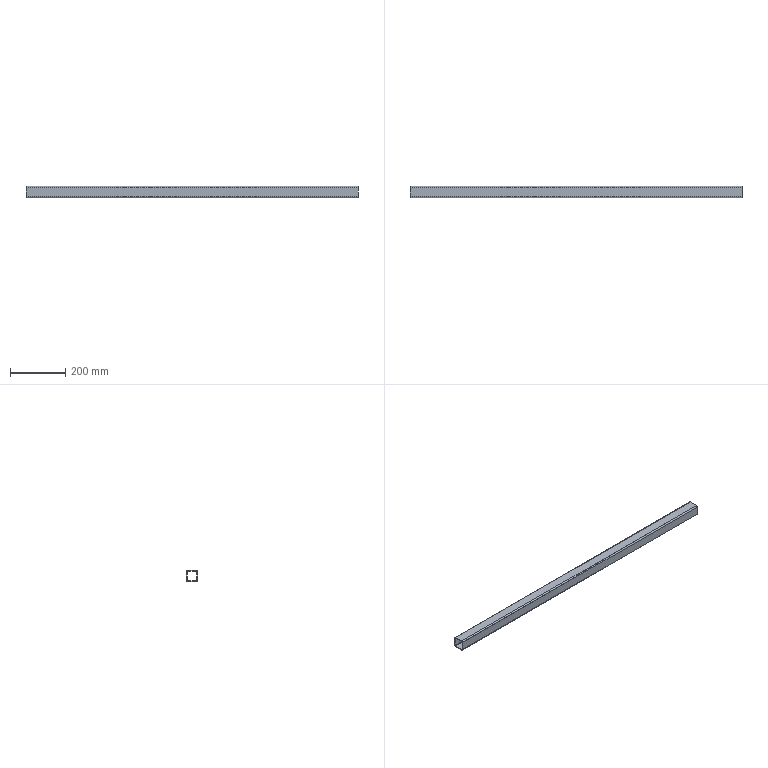Part | SolidWorks | features WeldMemberFeat 1, WeldmentFeature 1 | 1 solid | 18 faces | box 1200 x 40 x 40 mm | volume 399860 mm3 | plane 10 | cylinder 8 | commonest cylinder face diameters 4.6 x4 9.2 x4
STEP:
#1=CARTESIAN_POINT('',(0.,20.,15.4));
#2=VERTEX_POINT('',#1);
#3=CARTESIAN_POINT('',(0.,15.4,20.));
#4=VERTEX_POINT('',#3);
#5=CARTESIAN_POINT('',(0.,15.4,15.4));
#6=DIRECTION('',(1.,0.,0.));
#7=DIRECTION('',(0.,0.,-1.));
#8=AXIS2_PLACEMENT_3D('',#5,#6,#7);
#9=CIRCLE('',#8,4.6);
#10=EDGE_CURVE('',#2,#4,#9,.T.);
#11=ORIENTED_EDGE('',*,*,#10,.T.);
#12=CARTESIAN_POINT('',(1200.,15.4,20.));
#13=VERTEX_POINT('',#12);
#14=CARTESIAN_POINT('',(1200.,15.4,20.));
#15=DIRECTION('',(-1.,0.,0.));
#16=VECTOR('',#15,1000.);
#17=LINE('',#14,#16);
#18=EDGE_CURVE('',#13,#4,#17,.T.);
#19=ORIENTED_EDGE('',*,*,#18,.F.);
#20=CARTESIAN_POINT('',(1200.,20.,15.4));
#21=VERTEX_POINT('',#20);
#22=CARTESIAN_POINT('',(1200.,15.4,15.4));
#23=DIRECTION('',(1.,0.,0.));
#24=DIRECTION('',(0.,0.,-1.));
#25=AXIS2_PLACEMENT_3D('',#22,#23,#24);
#26=CIRCLE('',#25,4.6);
#27=EDGE_CURVE('',#21,#13,#26,.T.);
#28=ORIENTED_EDGE('',*,*,#27,.F.);
#29=CARTESIAN_POINT('',(1200.,20.,15.4));
#30=DIRECTION('',(-1.,0.,0.));
#31=VECTOR('',#30,1000.);
#32=LINE('',#29,#31);
#33=EDGE_CURVE('',#21,#2,#32,.T.);
#34=ORIENTED_EDGE('',*,*,#33,.T.);
#35=EDGE_LOOP('',(#11,#19,#28,#34));
#36=FACE_OUTER_BOUND('',#35,.T.);
#37=CARTESIAN_POINT('',(1200.,15.4,15.4));
#38=DIRECTION('',(-1.,0.,0.));
#39=DIRECTION('',(0.,0.,1.));
#40=AXIS2_PLACEMENT_3D('',#37,#38,#39);
#41=CYLINDRICAL_SURFACE('',#40,4.6);
#42=ADVANCED_FACE('',(#36),#41,.T.);
#43=CARTESIAN_POINT('',(0.,-15.4,20.));
#44=VERTEX_POINT('',#43);
#45=CARTESIAN_POINT('',(0.,15.4,20.));
#46=DIRECTION('',(0.,-1.,0.));
#47=VECTOR('',#46,1000.);
#48=LINE('',#45,#47);
#49=EDGE_CURVE('',#4,#44,#48,.T.);
#50=ORIENTED_EDGE('',*,*,#49,.T.);
#51=CARTESIAN_POINT('',(1200.,-15.4,20.));
#52=VERTEX_POINT('',#51);
#53=CARTESIAN_POINT('',(1200.,-15.4,20.));
#54=DIRECTION('',(-1.,0.,0.));
#55=VECTOR('',#54,1000.);
#56=LINE('',#53,#55);
#57=EDGE_CURVE('',#52,#44,#56,.T.);
#58=ORIENTED_EDGE('',*,*,#57,.F.);
#59=CARTESIAN_POINT('',(1200.,15.4,20.));
#60=DIRECTION('',(0.,-1.,0.));
#61=VECTOR('',#60,1000.);
#62=LINE('',#59,#61);
#63=EDGE_CURVE('',#13,#52,#62,.T.);
#64=ORIENTED_EDGE('',*,*,#63,.F.);
#65=ORIENTED_EDGE('',*,*,#18,.T.);
#66=EDGE_LOOP('',(#50,#58,#64,#65));
#67=FACE_OUTER_BOUND('',#66,.T.);
#68=CARTESIAN_POINT('',(1200.,15.4,20.));
#69=DIRECTION('',(0.,0.,-1.));
#70=DIRECTION('',(0.,1.,0.));
#71=AXIS2_PLACEMENT_3D('',#68,#69,#70);
#72=PLANE('',#71);
#73=ADVANCED_FACE('',(#67),#72,.F.);
#74=CARTESIAN_POINT('',(0.,-20.,15.4));
#75=VERTEX_POINT('',#74);
#76=CARTESIAN_POINT('',(0.,-15.4,15.4));
#77=DIRECTION('',(1.,0.,0.));
#78=DIRECTION('',(0.,0.,-1.));
#79=AXIS2_PLACEMENT_3D('',#76,#77,#78);
#80=CIRCLE('',#79,4.6);
#81=EDGE_CURVE('',#44,#75,#80,.T.);
#82=ORIENTED_EDGE('',*,*,#81,.T.);
#83=CARTESIAN_POINT('',(1200.,-20.,15.4));
#84=VERTEX_POINT('',#83);
#85=CARTESIAN_POINT('',(1200.,-20.,15.4));
#86=DIRECTION('',(-1.,0.,0.));
#87=VECTOR('',#86,1000.);
#88=LINE('',#85,#87);
#89=EDGE_CURVE('',#84,#75,#88,.T.);
#90=ORIENTED_EDGE('',*,*,#89,.F.);
#91=CARTESIAN_POINT('',(1200.,-15.4,15.4));
#92=DIRECTION('',(1.,0.,0.));
#93=DIRECTION('',(0.,0.,-1.));
#94=AXIS2_PLACEMENT_3D('',#91,#92,#93);
#95=CIRCLE('',#94,4.6);
#96=EDGE_CURVE('',#52,#84,#95,.T.);
#97=ORIENTED_EDGE('',*,*,#96,.F.);
#98=ORIENTED_EDGE('',*,*,#57,.T.);
#99=EDGE_LOOP('',(#82,#90,#97,#98));
#100=FACE_OUTER_BOUND('',#99,.T.);
#101=CARTESIAN_POINT('',(1200.,-15.4,15.4));
#102=DIRECTION('',(-1.,0.,0.));
#103=DIRECTION('',(0.,0.,1.));
#104=AXIS2_PLACEMENT_3D('',#101,#102,#103);
#105=CYLINDRICAL_SURFACE('',#104,4.6);
#106=ADVANCED_FACE('',(#100),#105,.T.);
#107=CARTESIAN_POINT('',(0.,-20.,-15.4));
#108=VERTEX_POINT('',#107);
#109=CARTESIAN_POINT('',(0.,-20.,-15.4));
#110=DIRECTION('',(0.,0.,-1.));
#111=VECTOR('',#110,1000.);
#112=LINE('',#109,#111);
#113=EDGE_CURVE('',#75,#108,#112,.T.);
#114=ORIENTED_EDGE('',*,*,#113,.T.);
#115=CARTESIAN_POINT('',(1200.,-20.,-15.4));
#116=VERTEX_POINT('',#115);
#117=CARTESIAN_POINT('',(1200.,-20.,-15.4));
#118=DIRECTION('',(-1.,0.,0.));
#119=VECTOR('',#118,1000.);
#120=LINE('',#117,#119);
#121=EDGE_CURVE('',#116,#108,#120,.T.);
#122=ORIENTED_EDGE('',*,*,#121,.F.);
#123=CARTESIAN_POINT('',(1200.,-20.,-15.4));
#124=DIRECTION('',(0.,0.,-1.));
#125=VECTOR('',#124,1000.);
#126=LINE('',#123,#125);
#127=EDGE_CURVE('',#84,#116,#126,.T.);
#128=ORIENTED_EDGE('',*,*,#127,.F.);
#129=ORIENTED_EDGE('',*,*,#89,.T.);
#130=EDGE_LOOP('',(#114,#122,#128,#129));
#131=FACE_OUTER_BOUND('',#130,.T.);
#132=CARTESIAN_POINT('',(1200.,-20.,-15.4));
#133=DIRECTION('',(0.,1.,0.));
#134=DIRECTION('',(0.,0.,1.));
#135=AXIS2_PLACEMENT_3D('',#132,#133,#134);
#136=PLANE('',#135);
#137=ADVANCED_FACE('',(#131),#136,.F.);
#138=CARTESIAN_POINT('',(0.,-15.4,-20.));
#139=VERTEX_POINT('',#138);
#140=CARTESIAN_POINT('',(0.,-15.4,-15.4));
#141=DIRECTION('',(1.,0.,0.));
#142=DIRECTION('',(0.,0.,-1.));
#143=AXIS2_PLACEMENT_3D('',#140,#141,#142);
#144=CIRCLE('',#143,4.6);
#145=EDGE_CURVE('',#108,#139,#144,.T.);
#146=ORIENTED_EDGE('',*,*,#145,.T.);
#147=CARTESIAN_POINT('',(1200.,-15.4,-20.));
#148=VERTEX_POINT('',#147);
#149=CARTESIAN_POINT('',(1200.,-15.4,-20.));
#150=DIRECTION('',(-1.,0.,0.));
#151=VECTOR('',#150,1000.);
#152=LINE('',#149,#151);
#153=EDGE_CURVE('',#148,#139,#152,.T.);
#154=ORIENTED_EDGE('',*,*,#153,.F.);
#155=CARTESIAN_POINT('',(1200.,-15.4,-15.4));
#156=DIRECTION('',(1.,0.,0.));
#157=DIRECTION('',(0.,0.,-1.));
#158=AXIS2_PLACEMENT_3D('',#155,#156,#157);
#159=CIRCLE('',#158,4.6);
#160=EDGE_CURVE('',#116,#148,#159,.T.);
#161=ORIENTED_EDGE('',*,*,#160,.F.);
#162=ORIENTED_EDGE('',*,*,#121,.T.);
#163=EDGE_LOOP('',(#146,#154,#161,#162));
#164=FACE_OUTER_BOUND('',#163,.T.);
#165=CARTESIAN_POINT('',(1200.,-15.4,-15.4));
#166=DIRECTION('',(-1.,0.,0.));
#167=DIRECTION('',(0.,0.,1.));
#168=AXIS2_PLACEMENT_3D('',#165,#166,#167);
#169=CYLINDRICAL_SURFACE('',#168,4.6);
#170=ADVANCED_FACE('',(#164),#169,.T.);
#171=CARTESIAN_POINT('',(0.,15.4,-20.));
#172=VERTEX_POINT('',#171);
#173=CARTESIAN_POINT('',(0.,-15.4,-20.));
#174=DIRECTION('',(0.,1.,0.));
#175=VECTOR('',#174,1000.);
#176=LINE('',#173,#175);
#177=EDGE_CURVE('',#139,#172,#176,.T.);
#178=ORIENTED_EDGE('',*,*,#177,.T.);
#179=CARTESIAN_POINT('',(1200.,15.4,-20.));
#180=VERTEX_POINT('',#179);
#181=CARTESIAN_POINT('',(1200.,15.4,-20.));
#182=DIRECTION('',(-1.,0.,0.));
#183=VECTOR('',#182,1000.);
#184=LINE('',#181,#183);
#185=EDGE_CURVE('',#180,#172,#184,.T.);
#186=ORIENTED_EDGE('',*,*,#185,.F.);
#187=CARTESIAN_POINT('',(1200.,-15.4,-20.));
#188=DIRECTION('',(0.,1.,0.));
#189=VECTOR('',#188,1000.);
#190=LINE('',#187,#189);
#191=EDGE_CURVE('',#148,#180,#190,.T.);
#192=ORIENTED_EDGE('',*,*,#191,.F.);
#193=ORIENTED_EDGE('',*,*,#153,.T.);
#194=EDGE_LOOP('',(#178,#186,#192,#193));
#195=FACE_OUTER_BOUND('',#194,.T.);
#196=CARTESIAN_POINT('',(1200.,-15.4,-20.));
#197=DIRECTION('',(0.,0.,1.));
#198=DIRECTION('',(0.,-1.,0.));
#199=AXIS2_PLACEMENT_3D('',#196,#197,#198);
#200=PLANE('',#199);
#201=ADVANCED_FACE('',(#195),#200,.F.);
#202=CARTESIAN_POINT('',(0.,20.,-15.4));
#203=VERTEX_POINT('',#202);
#204=CARTESIAN_POINT('',(0.,15.4,-15.4));
#205=DIRECTION('',(1.,0.,0.));
#206=DIRECTION('',(0.,0.,-1.));
#207=AXIS2_PLACEMENT_3D('',#204,#205,#206);
#208=CIRCLE('',#207,4.6);
#209=EDGE_CURVE('',#172,#203,#208,.T.);
#210=ORIENTED_EDGE('',*,*,#209,.T.);
#211=CARTESIAN_POINT('',(1200.,20.,-15.4));
#212=VERTEX_POINT('',#211);
#213=CARTESIAN_POINT('',(1200.,20.,-15.4));
#214=DIRECTION('',(-1.,0.,0.));
#215=VECTOR('',#214,1000.);
#216=LINE('',#213,#215);
#217=EDGE_CURVE('',#212,#203,#216,.T.);
#218=ORIENTED_EDGE('',*,*,#217,.F.);
#219=CARTESIAN_POINT('',(1200.,15.4,-15.4));
#220=DIRECTION('',(1.,0.,0.));
#221=DIRECTION('',(0.,0.,-1.));
#222=AXIS2_PLACEMENT_3D('',#219,#220,#221);
#223=CIRCLE('',#222,4.6);
#224=EDGE_CURVE('',#180,#212,#223,.T.);
#225=ORIENTED_EDGE('',*,*,#224,.F.);
#226=ORIENTED_EDGE('',*,*,#185,.T.);
#227=EDGE_LOOP('',(#210,#218,#225,#226));
#228=FACE_OUTER_BOUND('',#227,.T.);
#229=CARTESIAN_POINT('',(1200.,15.4,-15.4));
#230=DIRECTION('',(-1.,0.,0.));
#231=DIRECTION('',(0.,0.,1.));
#232=AXIS2_PLACEMENT_3D('',#229,#230,#231);
#233=CYLINDRICAL_SURFACE('',#232,4.6);
#234=ADVANCED_FACE('',(#228),#233,.T.);
#235=CARTESIAN_POINT('',(0.,-15.4,17.7));
#236=VERTEX_POINT('',#235);
#237=CARTESIAN_POINT('',(0.,-17.7,15.4));
#238=VERTEX_POINT('',#237);
#239=CARTESIAN_POINT('',(0.,-15.4,15.4));
#240=DIRECTION('',(1.,0.,0.));
#241=DIRECTION('',(0.,0.,-1.));
#242=AXIS2_PLACEMENT_3D('',#239,#240,#241);
#243=CIRCLE('',#242,2.3);
#244=EDGE_CURVE('',#236,#238,#243,.T.);
#245=ORIENTED_EDGE('',*,*,#244,.F.);
#246=CARTESIAN_POINT('',(1200.,-15.4,17.7));
#247=VERTEX_POINT('',#246);
#248=CARTESIAN_POINT('',(1200.,-15.4,17.7));
#249=DIRECTION('',(-1.,0.,0.));
#250=VECTOR('',#249,1000.);
#251=LINE('',#248,#250);
#252=EDGE_CURVE('',#247,#236,#251,.T.);
#253=ORIENTED_EDGE('',*,*,#252,.F.);
#254=CARTESIAN_POINT('',(1200.,-17.7,15.4));
#255=VERTEX_POINT('',#254);
#256=CARTESIAN_POINT('',(1200.,-15.4,15.4));
#257=DIRECTION('',(1.,0.,0.));
#258=DIRECTION('',(0.,0.,-1.));
#259=AXIS2_PLACEMENT_3D('',#256,#257,#258);
#260=CIRCLE('',#259,2.3);
#261=EDGE_CURVE('',#247,#255,#260,.T.);
#262=ORIENTED_EDGE('',*,*,#261,.T.);
#263=CARTESIAN_POINT('',(1200.,-17.7,15.4));
#264=DIRECTION('',(-1.,0.,0.));
#265=VECTOR('',#264,1000.);
#266=LINE('',#263,#265);
#267=EDGE_CURVE('',#255,#238,#266,.T.);
#268=ORIENTED_EDGE('',*,*,#267,.T.);
#269=EDGE_LOOP('',(#245,#253,#262,#268));
#270=FACE_OUTER_BOUND('',#269,.T.);
#271=CARTESIAN_POINT('',(1200.,-15.4,15.4));
#272=DIRECTION('',(-1.,0.,0.));
#273=DIRECTION('',(0.,0.,1.));
#274=AXIS2_PLACEMENT_3D('',#271,#272,#273);
#275=CYLINDRICAL_SURFACE('',#274,2.3);
#276=ADVANCED_FACE('',(#270),#275,.F.);
#277=CARTESIAN_POINT('',(0.,15.4,17.7));
#278=VERTEX_POINT('',#277);
#279=CARTESIAN_POINT('',(0.,15.4,17.7));
#280=DIRECTION('',(0.,-1.,0.));
#281=VECTOR('',#280,1000.);
#282=LINE('',#279,#281);
#283=EDGE_CURVE('',#278,#236,#282,.T.);
#284=ORIENTED_EDGE('',*,*,#283,.F.);
#285=CARTESIAN_POINT('',(1200.,15.4,17.7));
#286=VERTEX_POINT('',#285);
#287=CARTESIAN_POINT('',(1200.,15.4,17.7));
#288=DIRECTION('',(-1.,0.,0.));
#289=VECTOR('',#288,1000.);
#290=LINE('',#287,#289);
#291=EDGE_CURVE('',#286,#278,#290,.T.);
#292=ORIENTED_EDGE('',*,*,#291,.F.);
#293=CARTESIAN_POINT('',(1200.,15.4,17.7));
#294=DIRECTION('',(0.,-1.,0.));
#295=VECTOR('',#294,1000.);
#296=LINE('',#293,#295);
#297=EDGE_CURVE('',#286,#247,#296,.T.);
#298=ORIENTED_EDGE('',*,*,#297,.T.);
#299=ORIENTED_EDGE('',*,*,#252,.T.);
#300=EDGE_LOOP('',(#284,#292,#298,#299));
#301=FACE_OUTER_BOUND('',#300,.T.);
#302=CARTESIAN_POINT('',(1200.,15.4,17.7));
#303=DIRECTION('',(0.,0.,-1.));
#304=DIRECTION('',(0.,1.,0.));
#305=AXIS2_PLACEMENT_3D('',#302,#303,#304);
#306=PLANE('',#305);
#307=ADVANCED_FACE('',(#301),#306,.T.);
#308=CARTESIAN_POINT('',(0.,17.7,15.4));
#309=VERTEX_POINT('',#308);
#310=CARTESIAN_POINT('',(0.,15.4,15.4));
#311=DIRECTION('',(1.,0.,0.));
#312=DIRECTION('',(0.,0.,-1.));
#313=AXIS2_PLACEMENT_3D('',#310,#311,#312);
#314=CIRCLE('',#313,2.3);
#315=EDGE_CURVE('',#309,#278,#314,.T.);
#316=ORIENTED_EDGE('',*,*,#315,.F.);
#317=CARTESIAN_POINT('',(1200.,17.7,15.4));
#318=VERTEX_POINT('',#317);
#319=CARTESIAN_POINT('',(1200.,17.7,15.4));
#320=DIRECTION('',(-1.,0.,0.));
#321=VECTOR('',#320,1000.);
#322=LINE('',#319,#321);
#323=EDGE_CURVE('',#318,#309,#322,.T.);
#324=ORIENTED_EDGE('',*,*,#323,.F.);
#325=CARTESIAN_POINT('',(1200.,15.4,15.4));
#326=DIRECTION('',(1.,0.,0.));
#327=DIRECTION('',(0.,0.,-1.));
#328=AXIS2_PLACEMENT_3D('',#325,#326,#327);
#329=CIRCLE('',#328,2.3);
#330=EDGE_CURVE('',#318,#286,#329,.T.);
#331=ORIENTED_EDGE('',*,*,#330,.T.);
#332=ORIENTED_EDGE('',*,*,#291,.T.);
#333=EDGE_LOOP('',(#316,#324,#331,#332));
#334=FACE_OUTER_BOUND('',#333,.T.);
#335=CARTESIAN_POINT('',(1200.,15.4,15.4));
#336=DIRECTION('',(-1.,0.,0.));
#337=DIRECTION('',(0.,0.,1.));
#338=AXIS2_PLACEMENT_3D('',#335,#336,#337);
#339=CYLINDRICAL_SURFACE('',#338,2.3);
#340=ADVANCED_FACE('',(#334),#339,.F.);
#341=CARTESIAN_POINT('',(0.,17.7,-15.4));
#342=VERTEX_POINT('',#341);
#343=CARTESIAN_POINT('',(0.,17.7,15.4));
#344=DIRECTION('',(0.,0.,1.));
#345=VECTOR('',#344,1000.);
#346=LINE('',#343,#345);
#347=EDGE_CURVE('',#342,#309,#346,.T.);
#348=ORIENTED_EDGE('',*,*,#347,.F.);
#349=CARTESIAN_POINT('',(1200.,17.7,-15.4));
#350=VERTEX_POINT('',#349);
#351=CARTESIAN_POINT('',(1200.,17.7,-15.4));
#352=DIRECTION('',(-1.,0.,0.));
#353=VECTOR('',#352,1000.);
#354=LINE('',#351,#353);
#355=EDGE_CURVE('',#350,#342,#354,.T.);
#356=ORIENTED_EDGE('',*,*,#355,.F.);
#357=CARTESIAN_POINT('',(1200.,17.7,15.4));
#358=DIRECTION('',(0.,0.,1.));
#359=VECTOR('',#358,1000.);
#360=LINE('',#357,#359);
#361=EDGE_CURVE('',#350,#318,#360,.T.);
#362=ORIENTED_EDGE('',*,*,#361,.T.);
#363=ORIENTED_EDGE('',*,*,#323,.T.);
#364=EDGE_LOOP('',(#348,#356,#362,#363));
#365=FACE_OUTER_BOUND('',#364,.T.);
#366=CARTESIAN_POINT('',(1200.,17.7,15.4));
#367=DIRECTION('',(0.,-1.,0.));
#368=DIRECTION('',(0.,0.,-1.));
#369=AXIS2_PLACEMENT_3D('',#366,#367,#368);
#370=PLANE('',#369);
#371=ADVANCED_FACE('',(#365),#370,.T.);
#372=CARTESIAN_POINT('',(0.,15.4,-17.7));
#373=VERTEX_POINT('',#372);
#374=CARTESIAN_POINT('',(0.,15.4,-15.4));
#375=DIRECTION('',(1.,0.,0.));
#376=DIRECTION('',(0.,0.,-1.));
#377=AXIS2_PLACEMENT_3D('',#374,#375,#376);
#378=CIRCLE('',#377,2.3);
#379=EDGE_CURVE('',#373,#342,#378,.T.);
#380=ORIENTED_EDGE('',*,*,#379,.F.);
#381=CARTESIAN_POINT('',(1200.,15.4,-17.7));
#382=VERTEX_POINT('',#381);
#383=CARTESIAN_POINT('',(1200.,15.4,-17.7));
#384=DIRECTION('',(-1.,0.,0.));
#385=VECTOR('',#384,1000.);
#386=LINE('',#383,#385);
#387=EDGE_CURVE('',#382,#373,#386,.T.);
#388=ORIENTED_EDGE('',*,*,#387,.F.);
#389=CARTESIAN_POINT('',(1200.,15.4,-15.4));
#390=DIRECTION('',(1.,0.,0.));
#391=DIRECTION('',(0.,0.,-1.));
#392=AXIS2_PLACEMENT_3D('',#389,#390,#391);
#393=CIRCLE('',#392,2.3);
#394=EDGE_CURVE('',#382,#350,#393,.T.);
#395=ORIENTED_EDGE('',*,*,#394,.T.);
#396=ORIENTED_EDGE('',*,*,#355,.T.);
#397=EDGE_LOOP('',(#380,#388,#395,#396));
#398=FACE_OUTER_BOUND('',#397,.T.);
#399=CARTESIAN_POINT('',(1200.,15.4,-15.4));
#400=DIRECTION('',(-1.,0.,0.));
#401=DIRECTION('',(0.,0.,1.));
#402=AXIS2_PLACEMENT_3D('',#399,#400,#401);
#403=CYLINDRICAL_SURFACE('',#402,2.3);
#404=ADVANCED_FACE('',(#398),#403,.F.);
#405=CARTESIAN_POINT('',(0.,-15.4,-17.7));
#406=VERTEX_POINT('',#405);
#407=CARTESIAN_POINT('',(0.,-15.4,-17.7));
#408=DIRECTION('',(0.,1.,0.));
#409=VECTOR('',#408,1000.);
#410=LINE('',#407,#409);
#411=EDGE_CURVE('',#406,#373,#410,.T.);
#412=ORIENTED_EDGE('',*,*,#411,.F.);
#413=CARTESIAN_POINT('',(1200.,-15.4,-17.7));
#414=VERTEX_POINT('',#413);
#415=CARTESIAN_POINT('',(1200.,-15.4,-17.7));
#416=DIRECTION('',(-1.,0.,0.));
#417=VECTOR('',#416,1000.);
#418=LINE('',#415,#417);
#419=EDGE_CURVE('',#414,#406,#418,.T.);
#420=ORIENTED_EDGE('',*,*,#419,.F.);
#421=CARTESIAN_POINT('',(1200.,-15.4,-17.7));
#422=DIRECTION('',(0.,1.,0.));
#423=VECTOR('',#422,1000.);
#424=LINE('',#421,#423);
#425=EDGE_CURVE('',#414,#382,#424,.T.);
#426=ORIENTED_EDGE('',*,*,#425,.T.);
#427=ORIENTED_EDGE('',*,*,#387,.T.);
#428=EDGE_LOOP('',(#412,#420,#426,#427));
#429=FACE_OUTER_BOUND('',#428,.T.);
#430=CARTESIAN_POINT('',(1200.,-15.4,-17.7));
#431=DIRECTION('',(0.,0.,1.));
#432=DIRECTION('',(0.,-1.,0.));
#433=AXIS2_PLACEMENT_3D('',#430,#431,#432);
#434=PLANE('',#433);
#435=ADVANCED_FACE('',(#429),#434,.T.);
#436=CARTESIAN_POINT('',(0.,-17.7,-15.4));
#437=VERTEX_POINT('',#436);
#438=CARTESIAN_POINT('',(0.,-15.4,-15.4));
#439=DIRECTION('',(1.,0.,0.));
#440=DIRECTION('',(0.,0.,-1.));
#441=AXIS2_PLACEMENT_3D('',#438,#439,#440);
#442=CIRCLE('',#441,2.3);
#443=EDGE_CURVE('',#437,#406,#442,.T.);
#444=ORIENTED_EDGE('',*,*,#443,.F.);
#445=CARTESIAN_POINT('',(1200.,-17.7,-15.4));
#446=VERTEX_POINT('',#445);
#447=CARTESIAN_POINT('',(1200.,-17.7,-15.4));
#448=DIRECTION('',(-1.,0.,0.));
#449=VECTOR('',#448,1000.);
#450=LINE('',#447,#449);
#451=EDGE_CURVE('',#446,#437,#450,.T.);
#452=ORIENTED_EDGE('',*,*,#451,.F.);
#453=CARTESIAN_POINT('',(1200.,-15.4,-15.4));
#454=DIRECTION('',(1.,0.,0.));
#455=DIRECTION('',(0.,0.,-1.));
#456=AXIS2_PLACEMENT_3D('',#453,#454,#455);
#457=CIRCLE('',#456,2.3);
#458=EDGE_CURVE('',#446,#414,#457,.T.);
#459=ORIENTED_EDGE('',*,*,#458,.T.);
#460=ORIENTED_EDGE('',*,*,#419,.T.);
#461=EDGE_LOOP('',(#444,#452,#459,#460));
#462=FACE_OUTER_BOUND('',#461,.T.);
#463=CARTESIAN_POINT('',(1200.,-15.4,-15.4));
#464=DIRECTION('',(-1.,0.,0.));
#465=DIRECTION('',(0.,0.,1.));
#466=AXIS2_PLACEMENT_3D('',#463,#464,#465);
#467=CYLINDRICAL_SURFACE('',#466,2.3);
#468=ADVANCED_FACE('',(#462),#467,.F.);
#469=CARTESIAN_POINT('',(0.,-17.7,-15.4));
#470=DIRECTION('',(0.,0.,-1.));
#471=VECTOR('',#470,1000.);
#472=LINE('',#469,#471);
#473=EDGE_CURVE('',#238,#437,#472,.T.);
#474=ORIENTED_EDGE('',*,*,#473,.F.);
#475=ORIENTED_EDGE('',*,*,#267,.F.);
#476=CARTESIAN_POINT('',(1200.,-17.7,-15.4));
#477=DIRECTION('',(0.,0.,-1.));
#478=VECTOR('',#477,1000.);
#479=LINE('',#476,#478);
#480=EDGE_CURVE('',#255,#446,#479,.T.);
#481=ORIENTED_EDGE('',*,*,#480,.T.);
#482=ORIENTED_EDGE('',*,*,#451,.T.);
#483=EDGE_LOOP('',(#474,#475,#481,#482));
#484=FACE_OUTER_BOUND('',#483,.T.);
#485=CARTESIAN_POINT('',(1200.,-17.7,-15.4));
#486=DIRECTION('',(0.,1.,0.));
#487=DIRECTION('',(0.,0.,1.));
#488=AXIS2_PLACEMENT_3D('',#485,#486,#487);
#489=PLANE('',#488);
#490=ADVANCED_FACE('',(#484),#489,.T.);
#491=CARTESIAN_POINT('',(0.,20.,15.4));
#492=DIRECTION('',(0.,0.,1.));
#493=VECTOR('',#492,1000.);
#494=LINE('',#491,#493);
#495=EDGE_CURVE('',#203,#2,#494,.T.);
#496=ORIENTED_EDGE('',*,*,#495,.T.);
#497=ORIENTED_EDGE('',*,*,#33,.F.);
#498=CARTESIAN_POINT('',(1200.,20.,15.4));
#499=DIRECTION('',(0.,0.,1.));
#500=VECTOR('',#499,1000.);
#501=LINE('',#498,#500);
#502=EDGE_CURVE('',#212,#21,#501,.T.);
#503=ORIENTED_EDGE('',*,*,#502,.F.);
#504=ORIENTED_EDGE('',*,*,#217,.T.);
#505=EDGE_LOOP('',(#496,#497,#503,#504));
#506=FACE_OUTER_BOUND('',#505,.T.);
#507=CARTESIAN_POINT('',(1200.,20.,15.4));
#508=DIRECTION('',(0.,-1.,0.));
#509=DIRECTION('',(0.,0.,-1.));
#510=AXIS2_PLACEMENT_3D('',#507,#508,#509);
#511=PLANE('',#510);
#512=ADVANCED_FACE('',(#506),#511,.F.);
#513=ORIENTED_EDGE('',*,*,#261,.F.);
#514=ORIENTED_EDGE('',*,*,#297,.F.);
#515=ORIENTED_EDGE('',*,*,#330,.F.);
#516=ORIENTED_EDGE('',*,*,#361,.F.);
#517=ORIENTED_EDGE('',*,*,#394,.F.);
#518=ORIENTED_EDGE('',*,*,#425,.F.);
#519=ORIENTED_EDGE('',*,*,#458,.F.);
#520=ORIENTED_EDGE('',*,*,#480,.F.);
#521=EDGE_LOOP('',(#513,#514,#515,#516,#517,#518,#519,#520));
#522=FACE_BOUND('',#521,.T.);
#523=ORIENTED_EDGE('',*,*,#27,.T.);
#524=ORIENTED_EDGE('',*,*,#63,.T.);
#525=ORIENTED_EDGE('',*,*,#96,.T.);
#526=ORIENTED_EDGE('',*,*,#127,.T.);
#527=ORIENTED_EDGE('',*,*,#160,.T.);
#528=ORIENTED_EDGE('',*,*,#191,.T.);
#529=ORIENTED_EDGE('',*,*,#224,.T.);
#530=ORIENTED_EDGE('',*,*,#502,.T.);
#531=EDGE_LOOP('',(#523,#524,#525,#526,#527,#528,#529,#530));
#532=FACE_OUTER_BOUND('',#531,.T.);
#533=CARTESIAN_POINT('',(1200.,15.4,15.4));
#534=DIRECTION('',(1.,0.,0.));
#535=DIRECTION('',(0.,0.,-1.));
#536=AXIS2_PLACEMENT_3D('',#533,#534,#535);
#537=PLANE('',#536);
#538=ADVANCED_FACE('',(#522,#532),#537,.T.);
#539=ORIENTED_EDGE('',*,*,#244,.T.);
#540=ORIENTED_EDGE('',*,*,#473,.T.);
#541=ORIENTED_EDGE('',*,*,#443,.T.);
#542=ORIENTED_EDGE('',*,*,#411,.T.);
#543=ORIENTED_EDGE('',*,*,#379,.T.);
#544=ORIENTED_EDGE('',*,*,#347,.T.);
#545=ORIENTED_EDGE('',*,*,#315,.T.);
#546=ORIENTED_EDGE('',*,*,#283,.T.);
#547=EDGE_LOOP('',(#539,#540,#541,#542,#543,#544,#545,#546));
#548=FACE_BOUND('',#547,.T.);
#549=ORIENTED_EDGE('',*,*,#10,.F.);
#550=ORIENTED_EDGE('',*,*,#495,.F.);
#551=ORIENTED_EDGE('',*,*,#209,.F.);
#552=ORIENTED_EDGE('',*,*,#177,.F.);
#553=ORIENTED_EDGE('',*,*,#145,.F.);
#554=ORIENTED_EDGE('',*,*,#113,.F.);
#555=ORIENTED_EDGE('',*,*,#81,.F.);
#556=ORIENTED_EDGE('',*,*,#49,.F.);
#557=EDGE_LOOP('',(#549,#550,#551,#552,#553,#554,#555,#556));
#558=FACE_OUTER_BOUND('',#557,.T.);
#559=CARTESIAN_POINT('',(0.,15.4,15.4));
#560=DIRECTION('',(1.,0.,0.));
#561=DIRECTION('',(0.,0.,-1.));
#562=AXIS2_PLACEMENT_3D('',#559,#560,#561);
#563=PLANE('',#562);
#564=ADVANCED_FACE('',(#548,#558),#563,.F.);
#565=CLOSED_SHELL('',(#42,#73,#106,#137,#170,#201,#234,#276,#307,#340,#371,#404,#435,#468,#490,#512,#538,#564));
#566=MANIFOLD_SOLID_BREP('',#565);
#567=CARTESIAN_POINT('',(0.,0.,0.));
#568=DIRECTION('',(0.,0.,1.));
#569=DIRECTION('',(1.,0.,0.));
#570=AXIS2_PLACEMENT_3D('',#567,#568,#569);
#571=(LENGTH_UNIT()NAMED_UNIT(*)SI_UNIT(.MILLI.,.METRE.));
#572=UNCERTAINTY_MEASURE_WITH_UNIT(LENGTH_MEASURE(0.00001),#571,'','');
#573=(NAMED_UNIT(*)PLANE_ANGLE_UNIT()SI_UNIT($,.RADIAN.));
#574=(NAMED_UNIT(*)SI_UNIT($,.STERADIAN.)SOLID_ANGLE_UNIT());
#575=(GEOMETRIC_REPRESENTATION_CONTEXT(3)GLOBAL_UNCERTAINTY_ASSIGNED_CONTEXT((#572))GLOBAL_UNIT_ASSIGNED_CONTEXT((#571,#573,#574))REPRESENTATION_CONTEXT('',''));
#576=ADVANCED_BREP_SHAPE_REPRESENTATION('',(#566,#570),#575);